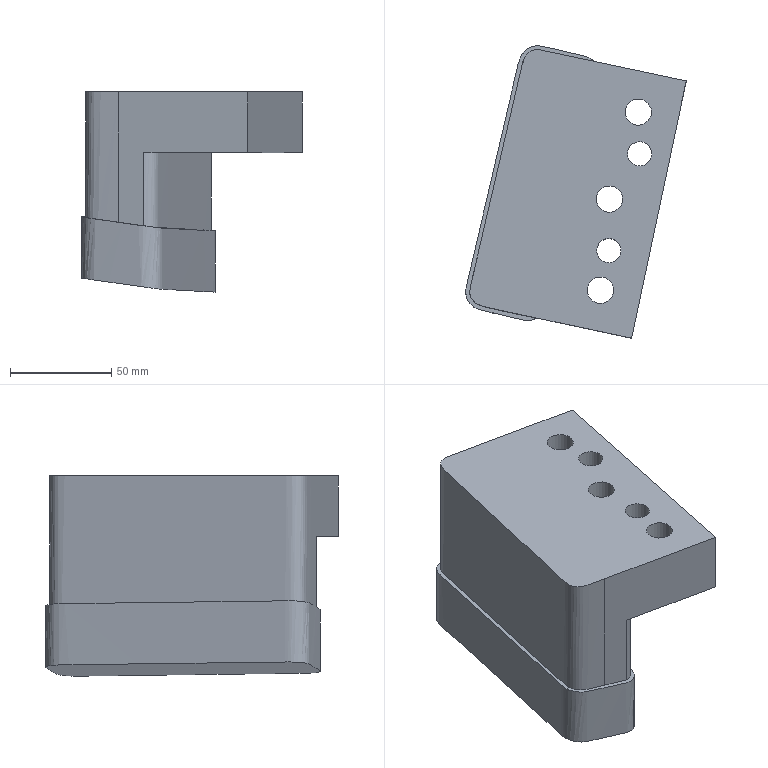Part | NX | features solid 2 | 1 solid | 21 faces | box 109.004 x 144.721 x 98.999 mm | volume 635341 mm3 | plane 8 | cylinder 8 | spline 5 | commonest cylinder face diameters 13 x3 20 x3 12 x2